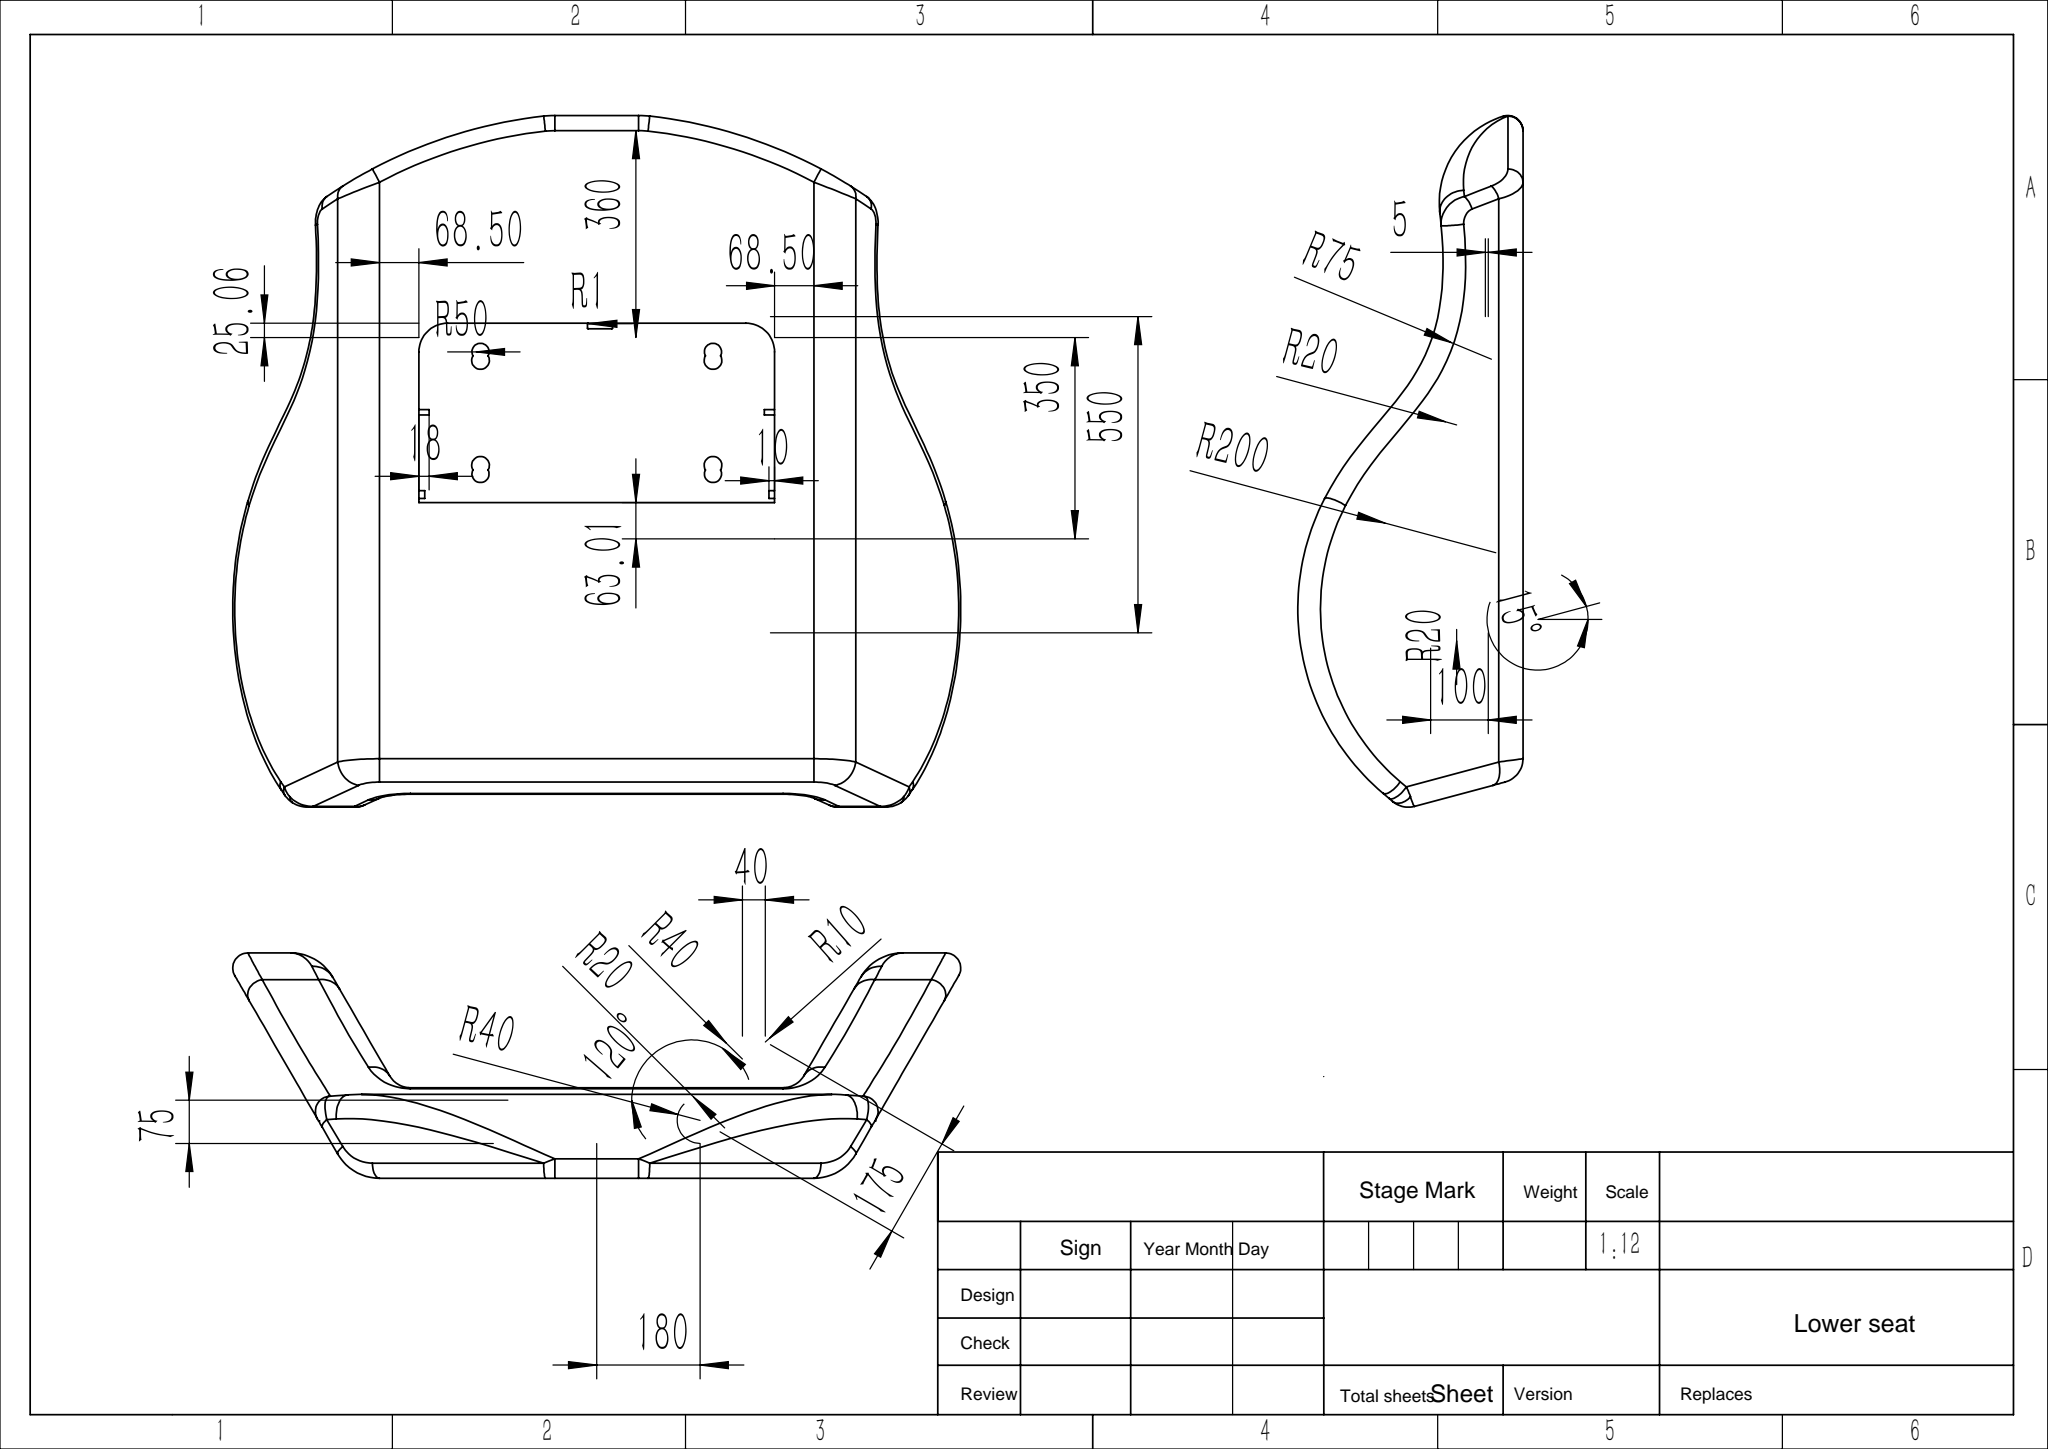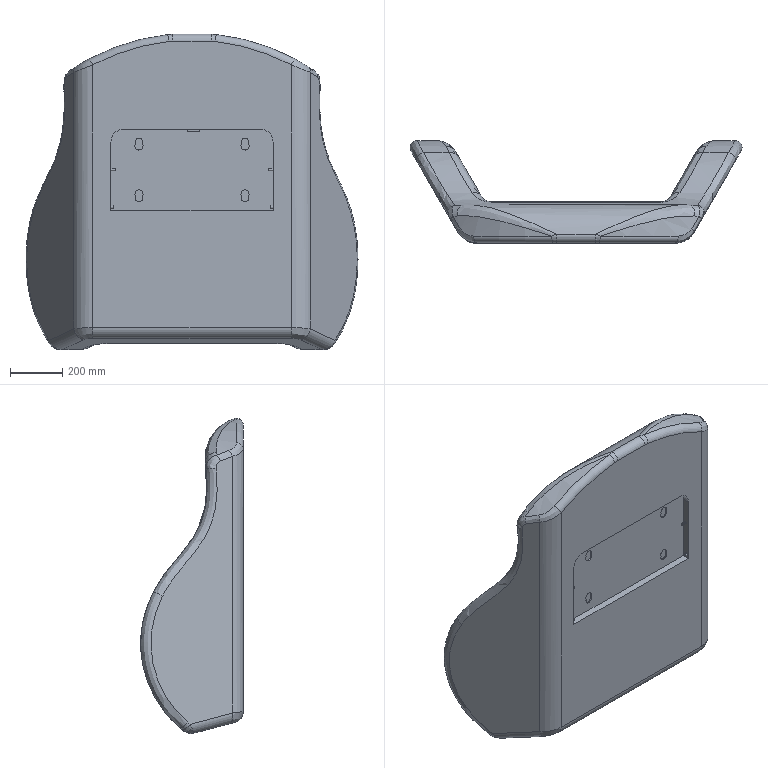Part | SolidWorks | features ICE 13, MirrorPattern 6, Fillet 5, Extrusion 1, RefAxis 1, Scale 1 | 1 solid | 133 faces | box 1267 x 391.764 x 1203 mm | volume 196548846 mm3 | cylinder 61 | spline 38 | plane 30 | torus 2 | sphere 2 | commonest cylinder face diameters 84 x15 29.779 x6 30.838 x6 2 x4 5 x4 5.2 x4